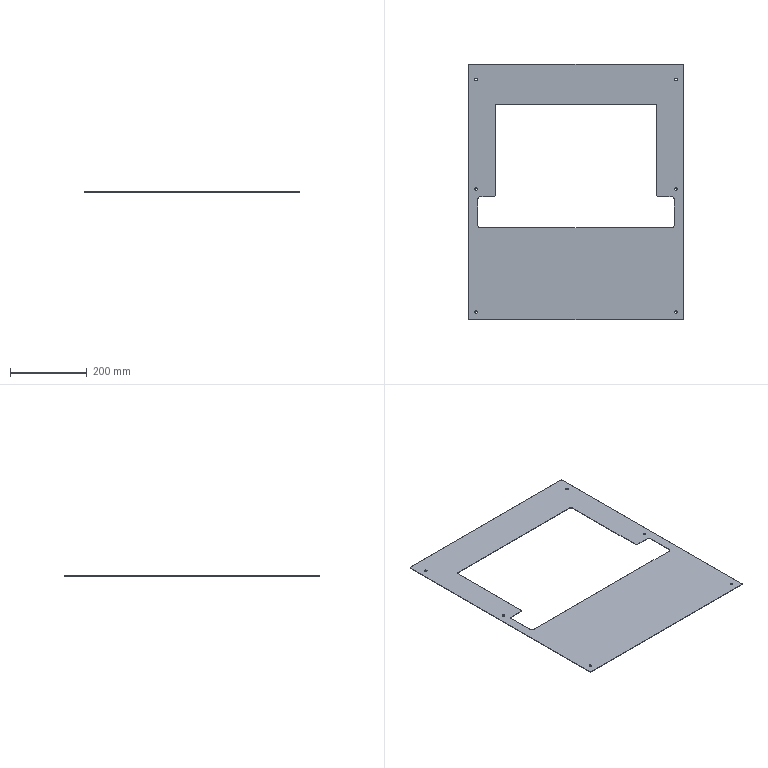Part | SolidWorks | features Fillet 2, ICE 2, FlatPattern 1, HoleWzd 1, SMBaseFlange 1, SheetMetal 1 | 1 solid | 38 faces | box 560 x 665 x 1.2 mm | volume 276730 mm3 | cylinder 24 | plane 14 | commonest cylinder face diameters 6.6 x12 10 x8 6 x4
STEP:
#1=CARTESIAN_POINT('',(16.7,-40.,0.));
#2=VERTEX_POINT('',#1);
#3=CARTESIAN_POINT('',(23.3,-40.,0.));
#4=VERTEX_POINT('',#3);
#5=CARTESIAN_POINT('',(20.,-40.,0.));
#6=DIRECTION('',(0.,0.,1.));
#7=DIRECTION('',(1.,0.,0.));
#8=AXIS2_PLACEMENT_3D('',#5,#6,#7);
#9=CIRCLE('',#8,3.3);
#10=EDGE_CURVE('',#2,#4,#9,.T.);
#11=ORIENTED_EDGE('',*,*,#10,.F.);
#12=CARTESIAN_POINT('',(16.7,-40.,1.2));
#13=VERTEX_POINT('',#12);
#14=CARTESIAN_POINT('',(16.7,-40.,1.2));
#15=DIRECTION('',(0.,0.,1.));
#16=VECTOR('',#15,1000.);
#17=LINE('',#14,#16);
#18=EDGE_CURVE('',#2,#13,#17,.T.);
#19=ORIENTED_EDGE('',*,*,#18,.T.);
#20=CARTESIAN_POINT('',(23.3,-40.,1.2));
#21=VERTEX_POINT('',#20);
#22=CARTESIAN_POINT('',(20.,-40.,1.2));
#23=DIRECTION('',(0.,0.,1.));
#24=DIRECTION('',(1.,0.,0.));
#25=AXIS2_PLACEMENT_3D('',#22,#23,#24);
#26=CIRCLE('',#25,3.3);
#27=EDGE_CURVE('',#13,#21,#26,.T.);
#28=ORIENTED_EDGE('',*,*,#27,.T.);
#29=CARTESIAN_POINT('',(23.3,-40.,1.2));
#30=DIRECTION('',(0.,0.,1.));
#31=VECTOR('',#30,1000.);
#32=LINE('',#29,#31);
#33=EDGE_CURVE('',#4,#21,#32,.T.);
#34=ORIENTED_EDGE('',*,*,#33,.F.);
#35=EDGE_LOOP('',(#11,#19,#28,#34));
#36=FACE_OUTER_BOUND('',#35,.T.);
#37=CARTESIAN_POINT('',(20.,-40.,1.2));
#38=DIRECTION('',(0.,0.,1.));
#39=DIRECTION('',(1.,0.,0.));
#40=AXIS2_PLACEMENT_3D('',#37,#38,#39);
#41=CYLINDRICAL_SURFACE('',#40,3.3);
#42=ADVANCED_FACE('',(#36),#41,.F.);
#43=CARTESIAN_POINT('',(536.7,-40.,0.));
#44=VERTEX_POINT('',#43);
#45=CARTESIAN_POINT('',(543.3,-40.,0.));
#46=VERTEX_POINT('',#45);
#47=CARTESIAN_POINT('',(540.,-40.,0.));
#48=DIRECTION('',(0.,0.,1.));
#49=DIRECTION('',(1.,0.,0.));
#50=AXIS2_PLACEMENT_3D('',#47,#48,#49);
#51=CIRCLE('',#50,3.3);
#52=EDGE_CURVE('',#44,#46,#51,.T.);
#53=ORIENTED_EDGE('',*,*,#52,.F.);
#54=CARTESIAN_POINT('',(536.7,-40.,1.2));
#55=VERTEX_POINT('',#54);
#56=CARTESIAN_POINT('',(536.7,-40.,1.2));
#57=DIRECTION('',(0.,0.,1.));
#58=VECTOR('',#57,1000.);
#59=LINE('',#56,#58);
#60=EDGE_CURVE('',#44,#55,#59,.T.);
#61=ORIENTED_EDGE('',*,*,#60,.T.);
#62=CARTESIAN_POINT('',(543.3,-40.,1.2));
#63=VERTEX_POINT('',#62);
#64=CARTESIAN_POINT('',(540.,-40.,1.2));
#65=DIRECTION('',(0.,0.,1.));
#66=DIRECTION('',(1.,0.,0.));
#67=AXIS2_PLACEMENT_3D('',#64,#65,#66);
#68=CIRCLE('',#67,3.3);
#69=EDGE_CURVE('',#55,#63,#68,.T.);
#70=ORIENTED_EDGE('',*,*,#69,.T.);
#71=CARTESIAN_POINT('',(543.3,-40.,1.2));
#72=DIRECTION('',(0.,0.,1.));
#73=VECTOR('',#72,1000.);
#74=LINE('',#71,#73);
#75=EDGE_CURVE('',#46,#63,#74,.T.);
#76=ORIENTED_EDGE('',*,*,#75,.F.);
#77=EDGE_LOOP('',(#53,#61,#70,#76));
#78=FACE_OUTER_BOUND('',#77,.T.);
#79=CARTESIAN_POINT('',(540.,-40.,1.2));
#80=DIRECTION('',(0.,0.,1.));
#81=DIRECTION('',(1.,0.,0.));
#82=AXIS2_PLACEMENT_3D('',#79,#80,#81);
#83=CYLINDRICAL_SURFACE('',#82,3.3);
#84=ADVANCED_FACE('',(#78),#83,.F.);
#85=CARTESIAN_POINT('',(16.7,-325.,0.));
#86=VERTEX_POINT('',#85);
#87=CARTESIAN_POINT('',(23.3,-325.,0.));
#88=VERTEX_POINT('',#87);
#89=CARTESIAN_POINT('',(20.,-325.,0.));
#90=DIRECTION('',(0.,0.,1.));
#91=DIRECTION('',(1.,0.,0.));
#92=AXIS2_PLACEMENT_3D('',#89,#90,#91);
#93=CIRCLE('',#92,3.3);
#94=EDGE_CURVE('',#86,#88,#93,.T.);
#95=ORIENTED_EDGE('',*,*,#94,.F.);
#96=CARTESIAN_POINT('',(16.7,-325.,1.2));
#97=VERTEX_POINT('',#96);
#98=CARTESIAN_POINT('',(16.7,-325.,1.2));
#99=DIRECTION('',(0.,0.,1.));
#100=VECTOR('',#99,1000.);
#101=LINE('',#98,#100);
#102=EDGE_CURVE('',#86,#97,#101,.T.);
#103=ORIENTED_EDGE('',*,*,#102,.T.);
#104=CARTESIAN_POINT('',(23.3,-325.,1.2));
#105=VERTEX_POINT('',#104);
#106=CARTESIAN_POINT('',(20.,-325.,1.2));
#107=DIRECTION('',(0.,0.,1.));
#108=DIRECTION('',(1.,0.,0.));
#109=AXIS2_PLACEMENT_3D('',#106,#107,#108);
#110=CIRCLE('',#109,3.3);
#111=EDGE_CURVE('',#97,#105,#110,.T.);
#112=ORIENTED_EDGE('',*,*,#111,.T.);
#113=CARTESIAN_POINT('',(23.3,-325.,1.2));
#114=DIRECTION('',(0.,0.,1.));
#115=VECTOR('',#114,1000.);
#116=LINE('',#113,#115);
#117=EDGE_CURVE('',#88,#105,#116,.T.);
#118=ORIENTED_EDGE('',*,*,#117,.F.);
#119=EDGE_LOOP('',(#95,#103,#112,#118));
#120=FACE_OUTER_BOUND('',#119,.T.);
#121=CARTESIAN_POINT('',(20.,-325.,1.2));
#122=DIRECTION('',(0.,0.,1.));
#123=DIRECTION('',(1.,0.,0.));
#124=AXIS2_PLACEMENT_3D('',#121,#122,#123);
#125=CYLINDRICAL_SURFACE('',#124,3.3);
#126=ADVANCED_FACE('',(#120),#125,.F.);
#127=CARTESIAN_POINT('',(536.7,-325.,0.));
#128=VERTEX_POINT('',#127);
#129=CARTESIAN_POINT('',(543.3,-325.,0.));
#130=VERTEX_POINT('',#129);
#131=CARTESIAN_POINT('',(540.,-325.,0.));
#132=DIRECTION('',(0.,0.,1.));
#133=DIRECTION('',(1.,0.,0.));
#134=AXIS2_PLACEMENT_3D('',#131,#132,#133);
#135=CIRCLE('',#134,3.3);
#136=EDGE_CURVE('',#128,#130,#135,.T.);
#137=ORIENTED_EDGE('',*,*,#136,.F.);
#138=CARTESIAN_POINT('',(536.7,-325.,1.2));
#139=VERTEX_POINT('',#138);
#140=CARTESIAN_POINT('',(536.7,-325.,1.2));
#141=DIRECTION('',(0.,0.,1.));
#142=VECTOR('',#141,1000.);
#143=LINE('',#140,#142);
#144=EDGE_CURVE('',#128,#139,#143,.T.);
#145=ORIENTED_EDGE('',*,*,#144,.T.);
#146=CARTESIAN_POINT('',(543.3,-325.,1.2));
#147=VERTEX_POINT('',#146);
#148=CARTESIAN_POINT('',(540.,-325.,1.2));
#149=DIRECTION('',(0.,0.,1.));
#150=DIRECTION('',(1.,0.,0.));
#151=AXIS2_PLACEMENT_3D('',#148,#149,#150);
#152=CIRCLE('',#151,3.3);
#153=EDGE_CURVE('',#139,#147,#152,.T.);
#154=ORIENTED_EDGE('',*,*,#153,.T.);
#155=CARTESIAN_POINT('',(543.3,-325.,1.2));
#156=DIRECTION('',(0.,0.,1.));
#157=VECTOR('',#156,1000.);
#158=LINE('',#155,#157);
#159=EDGE_CURVE('',#130,#147,#158,.T.);
#160=ORIENTED_EDGE('',*,*,#159,.F.);
#161=EDGE_LOOP('',(#137,#145,#154,#160));
#162=FACE_OUTER_BOUND('',#161,.T.);
#163=CARTESIAN_POINT('',(540.,-325.,1.2));
#164=DIRECTION('',(0.,0.,1.));
#165=DIRECTION('',(1.,0.,0.));
#166=AXIS2_PLACEMENT_3D('',#163,#164,#165);
#167=CYLINDRICAL_SURFACE('',#166,3.3);
#168=ADVANCED_FACE('',(#162),#167,.F.);
#169=CARTESIAN_POINT('',(16.7,-645.,0.));
#170=VERTEX_POINT('',#169);
#171=CARTESIAN_POINT('',(23.3,-645.,0.));
#172=VERTEX_POINT('',#171);
#173=CARTESIAN_POINT('',(20.,-645.,0.));
#174=DIRECTION('',(0.,0.,1.));
#175=DIRECTION('',(1.,0.,0.));
#176=AXIS2_PLACEMENT_3D('',#173,#174,#175);
#177=CIRCLE('',#176,3.3);
#178=EDGE_CURVE('',#170,#172,#177,.T.);
#179=ORIENTED_EDGE('',*,*,#178,.F.);
#180=CARTESIAN_POINT('',(16.7,-645.,1.2));
#181=VERTEX_POINT('',#180);
#182=CARTESIAN_POINT('',(16.7,-645.,1.2));
#183=DIRECTION('',(0.,0.,1.));
#184=VECTOR('',#183,1000.);
#185=LINE('',#182,#184);
#186=EDGE_CURVE('',#170,#181,#185,.T.);
#187=ORIENTED_EDGE('',*,*,#186,.T.);
#188=CARTESIAN_POINT('',(23.3,-645.,1.2));
#189=VERTEX_POINT('',#188);
#190=CARTESIAN_POINT('',(20.,-645.,1.2));
#191=DIRECTION('',(0.,0.,1.));
#192=DIRECTION('',(1.,0.,0.));
#193=AXIS2_PLACEMENT_3D('',#190,#191,#192);
#194=CIRCLE('',#193,3.3);
#195=EDGE_CURVE('',#181,#189,#194,.T.);
#196=ORIENTED_EDGE('',*,*,#195,.T.);
#197=CARTESIAN_POINT('',(23.3,-645.,1.2));
#198=DIRECTION('',(0.,0.,1.));
#199=VECTOR('',#198,1000.);
#200=LINE('',#197,#199);
#201=EDGE_CURVE('',#172,#189,#200,.T.);
#202=ORIENTED_EDGE('',*,*,#201,.F.);
#203=EDGE_LOOP('',(#179,#187,#196,#202));
#204=FACE_OUTER_BOUND('',#203,.T.);
#205=CARTESIAN_POINT('',(20.,-645.,1.2));
#206=DIRECTION('',(0.,0.,1.));
#207=DIRECTION('',(1.,0.,0.));
#208=AXIS2_PLACEMENT_3D('',#205,#206,#207);
#209=CYLINDRICAL_SURFACE('',#208,3.3);
#210=ADVANCED_FACE('',(#204),#209,.F.);
#211=CARTESIAN_POINT('',(536.7,-645.,0.));
#212=VERTEX_POINT('',#211);
#213=CARTESIAN_POINT('',(543.3,-645.,0.));
#214=VERTEX_POINT('',#213);
#215=CARTESIAN_POINT('',(540.,-645.,0.));
#216=DIRECTION('',(0.,0.,1.));
#217=DIRECTION('',(1.,0.,0.));
#218=AXIS2_PLACEMENT_3D('',#215,#216,#217);
#219=CIRCLE('',#218,3.3);
#220=EDGE_CURVE('',#212,#214,#219,.T.);
#221=ORIENTED_EDGE('',*,*,#220,.F.);
#222=CARTESIAN_POINT('',(536.7,-645.,1.2));
#223=VERTEX_POINT('',#222);
#224=CARTESIAN_POINT('',(536.7,-645.,1.2));
#225=DIRECTION('',(0.,0.,1.));
#226=VECTOR('',#225,1000.);
#227=LINE('',#224,#226);
#228=EDGE_CURVE('',#212,#223,#227,.T.);
#229=ORIENTED_EDGE('',*,*,#228,.T.);
#230=CARTESIAN_POINT('',(543.3,-645.,1.2));
#231=VERTEX_POINT('',#230);
#232=CARTESIAN_POINT('',(540.,-645.,1.2));
#233=DIRECTION('',(0.,0.,1.));
#234=DIRECTION('',(1.,0.,0.));
#235=AXIS2_PLACEMENT_3D('',#232,#233,#234);
#236=CIRCLE('',#235,3.3);
#237=EDGE_CURVE('',#223,#231,#236,.T.);
#238=ORIENTED_EDGE('',*,*,#237,.T.);
#239=CARTESIAN_POINT('',(543.3,-645.,1.2));
#240=DIRECTION('',(0.,0.,1.));
#241=VECTOR('',#240,1000.);
#242=LINE('',#239,#241);
#243=EDGE_CURVE('',#214,#231,#242,.T.);
#244=ORIENTED_EDGE('',*,*,#243,.F.);
#245=EDGE_LOOP('',(#221,#229,#238,#244));
#246=FACE_OUTER_BOUND('',#245,.T.);
#247=CARTESIAN_POINT('',(540.,-645.,1.2));
#248=DIRECTION('',(0.,0.,1.));
#249=DIRECTION('',(1.,0.,0.));
#250=AXIS2_PLACEMENT_3D('',#247,#248,#249);
#251=CYLINDRICAL_SURFACE('',#250,3.3);
#252=ADVANCED_FACE('',(#246),#251,.F.);
#253=CARTESIAN_POINT('',(0.,-662.,1.2));
#254=VERTEX_POINT('',#253);
#255=CARTESIAN_POINT('',(0.,-3.,1.2));
#256=VERTEX_POINT('',#255);
#257=CARTESIAN_POINT('',(0.,0.,1.2));
#258=DIRECTION('',(0.,1.,0.));
#259=VECTOR('',#258,1000.);
#260=LINE('',#257,#259);
#261=EDGE_CURVE('',#254,#256,#260,.T.);
#262=ORIENTED_EDGE('',*,*,#261,.T.);
#263=CARTESIAN_POINT('',(0.,-3.,0.));
#264=VERTEX_POINT('',#263);
#265=CARTESIAN_POINT('',(0.,-3.,1.2));
#266=DIRECTION('',(0.,0.,-1.));
#267=VECTOR('',#266,1000.);
#268=LINE('',#265,#267);
#269=EDGE_CURVE('',#256,#264,#268,.T.);
#270=ORIENTED_EDGE('',*,*,#269,.T.);
#271=CARTESIAN_POINT('',(0.,-662.,0.));
#272=VERTEX_POINT('',#271);
#273=CARTESIAN_POINT('',(0.,0.,0.));
#274=DIRECTION('',(0.,1.,0.));
#275=VECTOR('',#274,1000.);
#276=LINE('',#273,#275);
#277=EDGE_CURVE('',#272,#264,#276,.T.);
#278=ORIENTED_EDGE('',*,*,#277,.F.);
#279=CARTESIAN_POINT('',(0.,-662.,1.2));
#280=DIRECTION('',(0.,0.,1.));
#281=VECTOR('',#280,1000.);
#282=LINE('',#279,#281);
#283=EDGE_CURVE('',#272,#254,#282,.T.);
#284=ORIENTED_EDGE('',*,*,#283,.T.);
#285=EDGE_LOOP('',(#262,#270,#278,#284));
#286=FACE_OUTER_BOUND('',#285,.T.);
#287=CARTESIAN_POINT('',(0.,0.,1.2));
#288=DIRECTION('',(-1.,0.,0.));
#289=DIRECTION('',(0.,0.,1.));
#290=AXIS2_PLACEMENT_3D('',#287,#288,#289);
#291=PLANE('',#290);
#292=ADVANCED_FACE('',(#286),#291,.T.);
#293=CARTESIAN_POINT('',(557.,-665.,0.));
#294=VERTEX_POINT('',#293);
#295=CARTESIAN_POINT('',(3.,-665.,0.));
#296=VERTEX_POINT('',#295);
#297=CARTESIAN_POINT('',(0.,-665.,0.));
#298=DIRECTION('',(-1.,0.,0.));
#299=VECTOR('',#298,1000.);
#300=LINE('',#297,#299);
#301=EDGE_CURVE('',#294,#296,#300,.T.);
#302=ORIENTED_EDGE('',*,*,#301,.F.);
#303=CARTESIAN_POINT('',(557.,-665.,1.2));
#304=VERTEX_POINT('',#303);
#305=CARTESIAN_POINT('',(557.,-665.,1.2));
#306=DIRECTION('',(0.,0.,1.));
#307=VECTOR('',#306,1000.);
#308=LINE('',#305,#307);
#309=EDGE_CURVE('',#294,#304,#308,.T.);
#310=ORIENTED_EDGE('',*,*,#309,.T.);
#311=CARTESIAN_POINT('',(3.,-665.,1.2));
#312=VERTEX_POINT('',#311);
#313=CARTESIAN_POINT('',(0.,-665.,1.2));
#314=DIRECTION('',(-1.,0.,0.));
#315=VECTOR('',#314,1000.);
#316=LINE('',#313,#315);
#317=EDGE_CURVE('',#304,#312,#316,.T.);
#318=ORIENTED_EDGE('',*,*,#317,.T.);
#319=CARTESIAN_POINT('',(3.,-665.,1.2));
#320=DIRECTION('',(0.,0.,-1.));
#321=VECTOR('',#320,1000.);
#322=LINE('',#319,#321);
#323=EDGE_CURVE('',#312,#296,#322,.T.);
#324=ORIENTED_EDGE('',*,*,#323,.T.);
#325=EDGE_LOOP('',(#302,#310,#318,#324));
#326=FACE_OUTER_BOUND('',#325,.T.);
#327=CARTESIAN_POINT('',(0.,-665.,1.2));
#328=DIRECTION('',(0.,-1.,0.));
#329=DIRECTION('',(0.,0.,-1.));
#330=AXIS2_PLACEMENT_3D('',#327,#328,#329);
#331=PLANE('',#330);
#332=ADVANCED_FACE('',(#326),#331,.T.);
#333=CARTESIAN_POINT('',(560.,-3.,0.));
#334=VERTEX_POINT('',#333);
#335=CARTESIAN_POINT('',(560.,-662.,0.));
#336=VERTEX_POINT('',#335);
#337=CARTESIAN_POINT('',(560.,0.,0.));
#338=DIRECTION('',(0.,-1.,0.));
#339=VECTOR('',#338,1000.);
#340=LINE('',#337,#339);
#341=EDGE_CURVE('',#334,#336,#340,.T.);
#342=ORIENTED_EDGE('',*,*,#341,.F.);
#343=CARTESIAN_POINT('',(560.,-3.,1.2));
#344=VERTEX_POINT('',#343);
#345=CARTESIAN_POINT('',(560.,-3.,1.2));
#346=DIRECTION('',(0.,0.,1.));
#347=VECTOR('',#346,1000.);
#348=LINE('',#345,#347);
#349=EDGE_CURVE('',#334,#344,#348,.T.);
#350=ORIENTED_EDGE('',*,*,#349,.T.);
#351=CARTESIAN_POINT('',(560.,-662.,1.2));
#352=VERTEX_POINT('',#351);
#353=CARTESIAN_POINT('',(560.,0.,1.2));
#354=DIRECTION('',(0.,-1.,0.));
#355=VECTOR('',#354,1000.);
#356=LINE('',#353,#355);
#357=EDGE_CURVE('',#344,#352,#356,.T.);
#358=ORIENTED_EDGE('',*,*,#357,.T.);
#359=CARTESIAN_POINT('',(560.,-662.,1.2));
#360=DIRECTION('',(0.,0.,-1.));
#361=VECTOR('',#360,1000.);
#362=LINE('',#359,#361);
#363=EDGE_CURVE('',#352,#336,#362,.T.);
#364=ORIENTED_EDGE('',*,*,#363,.T.);
#365=EDGE_LOOP('',(#342,#350,#358,#364));
#366=FACE_OUTER_BOUND('',#365,.T.);
#367=CARTESIAN_POINT('',(560.,0.,1.2));
#368=DIRECTION('',(1.,0.,0.));
#369=DIRECTION('',(0.,0.,-1.));
#370=AXIS2_PLACEMENT_3D('',#367,#368,#369);
#371=PLANE('',#370);
#372=ADVANCED_FACE('',(#366),#371,.T.);
#373=CARTESIAN_POINT('',(3.,0.,1.2));
#374=VERTEX_POINT('',#373);
#375=CARTESIAN_POINT('',(557.,0.,1.2));
#376=VERTEX_POINT('',#375);
#377=CARTESIAN_POINT('',(0.,0.,1.2));
#378=DIRECTION('',(1.,0.,0.));
#379=VECTOR('',#378,1000.);
#380=LINE('',#377,#379);
#381=EDGE_CURVE('',#374,#376,#380,.T.);
#382=ORIENTED_EDGE('',*,*,#381,.T.);
#383=CARTESIAN_POINT('',(557.,0.,0.));
#384=VERTEX_POINT('',#383);
#385=CARTESIAN_POINT('',(557.,0.,1.2));
#386=DIRECTION('',(0.,0.,-1.));
#387=VECTOR('',#386,1000.);
#388=LINE('',#385,#387);
#389=EDGE_CURVE('',#376,#384,#388,.T.);
#390=ORIENTED_EDGE('',*,*,#389,.T.);
#391=CARTESIAN_POINT('',(3.,0.,0.));
#392=VERTEX_POINT('',#391);
#393=CARTESIAN_POINT('',(0.,0.,0.));
#394=DIRECTION('',(1.,0.,0.));
#395=VECTOR('',#394,1000.);
#396=LINE('',#393,#395);
#397=EDGE_CURVE('',#392,#384,#396,.T.);
#398=ORIENTED_EDGE('',*,*,#397,.F.);
#399=CARTESIAN_POINT('',(3.,0.,1.2));
#400=DIRECTION('',(0.,0.,1.));
#401=VECTOR('',#400,1000.);
#402=LINE('',#399,#401);
#403=EDGE_CURVE('',#392,#374,#402,.T.);
#404=ORIENTED_EDGE('',*,*,#403,.T.);
#405=EDGE_LOOP('',(#382,#390,#398,#404));
#406=FACE_OUTER_BOUND('',#405,.T.);
#407=CARTESIAN_POINT('',(0.,0.,1.2));
#408=DIRECTION('',(0.,1.,0.));
#409=DIRECTION('',(0.,0.,1.));
#410=AXIS2_PLACEMENT_3D('',#407,#408,#409);
#411=PLANE('',#410);
#412=ADVANCED_FACE('',(#406),#411,.T.);
#413=CARTESIAN_POINT('',(20.,-40.,1.2));
#414=DIRECTION('',(0.,0.,1.));
#415=DIRECTION('',(1.,0.,0.));
#416=AXIS2_PLACEMENT_3D('',#413,#414,#415);
#417=CIRCLE('',#416,3.3);
#418=EDGE_CURVE('',#21,#13,#417,.T.);
#419=ORIENTED_EDGE('',*,*,#418,.F.);
#420=ORIENTED_EDGE('',*,*,#27,.F.);
#421=EDGE_LOOP('',(#419,#420));
#422=FACE_BOUND('',#421,.T.);
#423=CARTESIAN_POINT('',(540.,-40.,1.2));
#424=DIRECTION('',(0.,0.,1.));
#425=DIRECTION('',(1.,0.,0.));
#426=AXIS2_PLACEMENT_3D('',#423,#424,#425);
#427=CIRCLE('',#426,3.3);
#428=EDGE_CURVE('',#63,#55,#427,.T.);
#429=ORIENTED_EDGE('',*,*,#428,.F.);
#430=ORIENTED_EDGE('',*,*,#69,.F.);
#431=EDGE_LOOP('',(#429,#430));
#432=FACE_BOUND('',#431,.T.);
#433=CARTESIAN_POINT('',(20.,-325.,1.2));
#434=DIRECTION('',(0.,0.,1.));
#435=DIRECTION('',(1.,0.,0.));
#436=AXIS2_PLACEMENT_3D('',#433,#434,#435);
#437=CIRCLE('',#436,3.3);
#438=EDGE_CURVE('',#105,#97,#437,.T.);
#439=ORIENTED_EDGE('',*,*,#438,.F.);
#440=ORIENTED_EDGE('',*,*,#111,.F.);
#441=EDGE_LOOP('',(#439,#440));
#442=FACE_BOUND('',#441,.T.);
#443=CARTESIAN_POINT('',(540.,-325.,1.2));
#444=DIRECTION('',(0.,0.,1.));
#445=DIRECTION('',(1.,0.,0.));
#446=AXIS2_PLACEMENT_3D('',#443,#444,#445);
#447=CIRCLE('',#446,3.3);
#448=EDGE_CURVE('',#147,#139,#447,.T.);
#449=ORIENTED_EDGE('',*,*,#448,.F.);
#450=ORIENTED_EDGE('',*,*,#153,.F.);
#451=EDGE_LOOP('',(#449,#450));
#452=FACE_BOUND('',#451,.T.);
#453=CARTESIAN_POINT('',(20.,-645.,1.2));
#454=DIRECTION('',(0.,0.,1.));
#455=DIRECTION('',(1.,0.,0.));
#456=AXIS2_PLACEMENT_3D('',#453,#454,#455);
#457=CIRCLE('',#456,3.3);
#458=EDGE_CURVE('',#189,#181,#457,.T.);
#459=ORIENTED_EDGE('',*,*,#458,.F.);
#460=ORIENTED_EDGE('',*,*,#195,.F.);
#461=EDGE_LOOP('',(#459,#460));
#462=FACE_BOUND('',#461,.T.);
#463=CARTESIAN_POINT('',(540.,-645.,1.2));
#464=DIRECTION('',(0.,0.,1.));
#465=DIRECTION('',(1.,0.,0.));
#466=AXIS2_PLACEMENT_3D('',#463,#464,#465);
#467=CIRCLE('',#466,3.3);
#468=EDGE_CURVE('',#231,#223,#467,.T.);
#469=ORIENTED_EDGE('',*,*,#468,.F.);
#470=ORIENTED_EDGE('',*,*,#237,.F.);
#471=EDGE_LOOP('',(#469,#470));
#472=FACE_BOUND('',#471,.T.);
#473=CARTESIAN_POINT('',(65.,-345.,1.2));
#474=VERTEX_POINT('',#473);
#475=CARTESIAN_POINT('',(30.,-345.,1.2));
#476=VERTEX_POINT('',#475);
#477=CARTESIAN_POINT('',(25.,-345.,1.2));
#478=DIRECTION('',(-1.,0.,0.));
#479=VECTOR('',#478,1000.);
#480=LINE('',#477,#479);
#481=EDGE_CURVE('',#474,#476,#480,.T.);
#482=ORIENTED_EDGE('',*,*,#481,.F.);
#483=CARTESIAN_POINT('',(70.,-340.,1.2));
#484=VERTEX_POINT('',#483);
#485=CARTESIAN_POINT('',(65.,-340.,1.2));
#486=DIRECTION('',(0.,0.,1.));
#487=DIRECTION('',(1.,0.,0.));
#488=AXIS2_PLACEMENT_3D('',#485,#486,#487);
#489=CIRCLE('',#488,5.);
#490=EDGE_CURVE('',#474,#484,#489,.T.);
#491=ORIENTED_EDGE('',*,*,#490,.T.);
#492=CARTESIAN_POINT('',(70.,-110.,1.2));
#493=VERTEX_POINT('',#492);
#494=CARTESIAN_POINT('',(70.,-105.,1.2));
#495=DIRECTION('',(0.,-1.,0.));
#496=VECTOR('',#495,1000.);
#497=LINE('',#494,#496);
#498=EDGE_CURVE('',#493,#484,#497,.T.);
#499=ORIENTED_EDGE('',*,*,#498,.F.);
#500=CARTESIAN_POINT('',(75.,-105.,1.2));
#501=VERTEX_POINT('',#500);
#502=CARTESIAN_POINT('',(75.,-110.,1.2));
#503=DIRECTION('',(0.,0.,-1.));
#504=DIRECTION('',(1.,0.,0.));
#505=AXIS2_PLACEMENT_3D('',#502,#503,#504);
#506=CIRCLE('',#505,5.);
#507=EDGE_CURVE('',#493,#501,#506,.T.);
#508=ORIENTED_EDGE('',*,*,#507,.T.);
#509=CARTESIAN_POINT('',(485.,-105.,1.2));
#510=VERTEX_POINT('',#509);
#511=CARTESIAN_POINT('',(70.,-105.,1.2));
#512=DIRECTION('',(-1.,0.,0.));
#513=VECTOR('',#512,1000.);
#514=LINE('',#511,#513);
#515=EDGE_CURVE('',#510,#501,#514,.T.);
#516=ORIENTED_EDGE('',*,*,#515,.F.);
#517=CARTESIAN_POINT('',(490.,-110.,1.2));
#518=VERTEX_POINT('',#517);
#519=CARTESIAN_POINT('',(485.,-110.,1.2));
#520=DIRECTION('',(0.,0.,-1.));
#521=DIRECTION('',(1.,0.,0.));
#522=AXIS2_PLACEMENT_3D('',#519,#520,#521);
#523=CIRCLE('',#522,5.);
#524=EDGE_CURVE('',#510,#518,#523,.T.);
#525=ORIENTED_EDGE('',*,*,#524,.T.);
#526=CARTESIAN_POINT('',(490.,-340.,1.2));
#527=VERTEX_POINT('',#526);
#528=CARTESIAN_POINT('',(490.,-105.,1.2));
#529=DIRECTION('',(0.,1.,0.));
#530=VECTOR('',#529,1000.);
#531=LINE('',#528,#530);
#532=EDGE_CURVE('',#527,#518,#531,.T.);
#533=ORIENTED_EDGE('',*,*,#532,.F.);
#534=CARTESIAN_POINT('',(495.,-345.,1.2));
#535=VERTEX_POINT('',#534);
#536=CARTESIAN_POINT('',(495.,-340.,1.2));
#537=DIRECTION('',(0.,0.,1.));
#538=DIRECTION('',(1.,0.,0.));
#539=AXIS2_PLACEMENT_3D('',#536,#537,#538);
#540=CIRCLE('',#539,5.);
#541=EDGE_CURVE('',#527,#535,#540,.T.);
#542=ORIENTED_EDGE('',*,*,#541,.T.);
#543=CARTESIAN_POINT('',(530.,-345.,1.2));
#544=VERTEX_POINT('',#543);
#545=CARTESIAN_POINT('',(25.,-345.,1.2));
#546=DIRECTION('',(-1.,0.,0.));
#547=VECTOR('',#546,1000.);
#548=LINE('',#545,#547);
#549=EDGE_CURVE('',#544,#535,#548,.T.);
#550=ORIENTED_EDGE('',*,*,#549,.F.);
#551=CARTESIAN_POINT('',(535.,-350.,1.2));
#552=VERTEX_POINT('',#551);
#553=CARTESIAN_POINT('',(530.,-350.,1.2));
#554=DIRECTION('',(0.,0.,-1.));
#555=DIRECTION('',(1.,0.,0.));
#556=AXIS2_PLACEMENT_3D('',#553,#554,#555);
#557=CIRCLE('',#556,5.);
#558=EDGE_CURVE('',#544,#552,#557,.T.);
#559=ORIENTED_EDGE('',*,*,#558,.T.);
#560=CARTESIAN_POINT('',(535.,-420.,1.2));
#561=VERTEX_POINT('',#560);
#562=CARTESIAN_POINT('',(535.,-345.,1.2));
#563=DIRECTION('',(0.,1.,0.));
#564=VECTOR('',#563,1000.);
#565=LINE('',#562,#564);
#566=EDGE_CURVE('',#561,#552,#565,.T.);
#567=ORIENTED_EDGE('',*,*,#566,.F.);
#568=CARTESIAN_POINT('',(530.,-425.,1.2));
#569=VERTEX_POINT('',#568);
#570=CARTESIAN_POINT('',(530.,-420.,1.2));
#571=DIRECTION('',(0.,0.,-1.));
#572=DIRECTION('',(1.,0.,0.));
#573=AXIS2_PLACEMENT_3D('',#570,#571,#572);
#574=CIRCLE('',#573,5.);
#575=EDGE_CURVE('',#561,#569,#574,.T.);
#576=ORIENTED_EDGE('',*,*,#575,.T.);
#577=CARTESIAN_POINT('',(30.,-425.,1.2));
#578=VERTEX_POINT('',#577);
#579=CARTESIAN_POINT('',(70.,-425.,1.2));
#580=DIRECTION('',(1.,0.,0.));
#581=VECTOR('',#580,1000.);
#582=LINE('',#579,#581);
#583=EDGE_CURVE('',#578,#569,#582,.T.);
#584=ORIENTED_EDGE('',*,*,#583,.F.);
#585=CARTESIAN_POINT('',(25.,-420.,1.2));
#586=VERTEX_POINT('',#585);
#587=CARTESIAN_POINT('',(30.,-420.,1.2));
#588=DIRECTION('',(0.,0.,-1.));
#589=DIRECTION('',(1.,0.,0.));
#590=AXIS2_PLACEMENT_3D('',#587,#588,#589);
#591=CIRCLE('',#590,5.);
#592=EDGE_CURVE('',#578,#586,#591,.T.);
#593=ORIENTED_EDGE('',*,*,#592,.T.);
#594=CARTESIAN_POINT('',(25.,-350.,1.2));
#595=VERTEX_POINT('',#594);
#596=CARTESIAN_POINT('',(25.,-345.,1.2));
#597=DIRECTION('',(0.,-1.,0.));
#598=VECTOR('',#597,1000.);
#599=LINE('',#596,#598);
#600=EDGE_CURVE('',#595,#586,#599,.T.);
#601=ORIENTED_EDGE('',*,*,#600,.F.);
#602=CARTESIAN_POINT('',(30.,-350.,1.2));
#603=DIRECTION('',(0.,0.,-1.));
#604=DIRECTION('',(1.,0.,0.));
#605=AXIS2_PLACEMENT_3D('',#602,#603,#604);
#606=CIRCLE('',#605,5.);
#607=EDGE_CURVE('',#595,#476,#606,.T.);
#608=ORIENTED_EDGE('',*,*,#607,.T.);
#609=EDGE_LOOP('',(#482,#491,#499,#508,#516,#525,#533,#542,#550,#559,#567,#576,#584,#593,#601,#608));
#610=FACE_BOUND('',#609,.T.);
#611=ORIENTED_EDGE('',*,*,#357,.F.);
#612=CARTESIAN_POINT('',(557.,-3.,1.2));
#613=DIRECTION('',(0.,0.,1.));
#614=DIRECTION('',(1.,0.,0.));
#615=AXIS2_PLACEMENT_3D('',#612,#613,#614);
#616=CIRCLE('',#615,3.);
#617=EDGE_CURVE('',#344,#376,#616,.T.);
#618=ORIENTED_EDGE('',*,*,#617,.T.);
#619=ORIENTED_EDGE('',*,*,#381,.F.);
#620=CARTESIAN_POINT('',(3.,-3.,1.2));
#621=DIRECTION('',(0.,0.,1.));
#622=DIRECTION('',(1.,0.,0.));
#623=AXIS2_PLACEMENT_3D('',#620,#621,#622);
#624=CIRCLE('',#623,3.);
#625=EDGE_CURVE('',#374,#256,#624,.T.);
#626=ORIENTED_EDGE('',*,*,#625,.T.);
#627=ORIENTED_EDGE('',*,*,#261,.F.);
#628=CARTESIAN_POINT('',(3.,-662.,1.2));
#629=DIRECTION('',(0.,0.,1.));
#630=DIRECTION('',(1.,0.,0.));
#631=AXIS2_PLACEMENT_3D('',#628,#629,#630);
#632=CIRCLE('',#631,3.);
#633=EDGE_CURVE('',#254,#312,#632,.T.);
#634=ORIENTED_EDGE('',*,*,#633,.T.);
#635=ORIENTED_EDGE('',*,*,#317,.F.);
#636=CARTESIAN_POINT('',(557.,-662.,1.2));
#637=DIRECTION('',(0.,0.,1.));
#638=DIRECTION('',(1.,0.,0.));
#639=AXIS2_PLACEMENT_3D('',#636,#637,#638);
#640=CIRCLE('',#639,3.);
#641=EDGE_CURVE('',#304,#352,#640,.T.);
#642=ORIENTED_EDGE('',*,*,#641,.T.);
#643=EDGE_LOOP('',(#611,#618,#619,#626,#627,#634,#635,#642));
#644=FACE_OUTER_BOUND('',#643,.T.);
#645=CARTESIAN_POINT('',(0.,0.,1.2));
#646=DIRECTION('',(0.,0.,1.));
#647=DIRECTION('',(1.,0.,0.));
#648=AXIS2_PLACEMENT_3D('',#645,#646,#647);
#649=PLANE('',#648);
#650=ADVANCED_FACE('',(#422,#432,#442,#452,#462,#472,#610,#644),#649,.T.);
#651=CARTESIAN_POINT('',(20.,-40.,0.));
#652=DIRECTION('',(0.,0.,1.));
#653=DIRECTION('',(1.,0.,0.));
#654=AXIS2_PLACEMENT_3D('',#651,#652,#653);
#655=CIRCLE('',#654,3.3);
#656=EDGE_CURVE('',#4,#2,#655,.T.);
#657=ORIENTED_EDGE('',*,*,#656,.T.);
#658=ORIENTED_EDGE('',*,*,#10,.T.);
#659=EDGE_LOOP('',(#657,#658));
#660=FACE_BOUND('',#659,.T.);
#661=CARTESIAN_POINT('',(540.,-40.,0.));
#662=DIRECTION('',(0.,0.,1.));
#663=DIRECTION('',(1.,0.,0.));
#664=AXIS2_PLACEMENT_3D('',#661,#662,#663);
#665=CIRCLE('',#664,3.3);
#666=EDGE_CURVE('',#46,#44,#665,.T.);
#667=ORIENTED_EDGE('',*,*,#666,.T.);
#668=ORIENTED_EDGE('',*,*,#52,.T.);
#669=EDGE_LOOP('',(#667,#668));
#670=FACE_BOUND('',#669,.T.);
#671=CARTESIAN_POINT('',(20.,-325.,0.));
#672=DIRECTION('',(0.,0.,1.));
#673=DIRECTION('',(1.,0.,0.));
#674=AXIS2_PLACEMENT_3D('',#671,#672,#673);
#675=CIRCLE('',#674,3.3);
#676=EDGE_CURVE('',#88,#86,#675,.T.);
#677=ORIENTED_EDGE('',*,*,#676,.T.);
#678=ORIENTED_EDGE('',*,*,#94,.T.);
#679=EDGE_LOOP('',(#677,#678));
#680=FACE_BOUND('',#679,.T.);
#681=CARTESIAN_POINT('',(540.,-325.,0.));
#682=DIRECTION('',(0.,0.,1.));
#683=DIRECTION('',(1.,0.,0.));
#684=AXIS2_PLACEMENT_3D('',#681,#682,#683);
#685=CIRCLE('',#684,3.3);
#686=EDGE_CURVE('',#130,#128,#685,.T.);
#687=ORIENTED_EDGE('',*,*,#686,.T.);
#688=ORIENTED_EDGE('',*,*,#136,.T.);
#689=EDGE_LOOP('',(#687,#688));
#690=FACE_BOUND('',#689,.T.);
#691=CARTESIAN_POINT('',(20.,-645.,0.));
#692=DIRECTION('',(0.,0.,1.));
#693=DIRECTION('',(1.,0.,0.));
#694=AXIS2_PLACEMENT_3D('',#691,#692,#693);
#695=CIRCLE('',#694,3.3);
#696=EDGE_CURVE('',#172,#170,#695,.T.);
#697=ORIENTED_EDGE('',*,*,#696,.T.);
#698=ORIENTED_EDGE('',*,*,#178,.T.);
#699=EDGE_LOOP('',(#697,#698));
#700=FACE_BOUND('',#699,.T.);
#701=CARTESIAN_POINT('',(540.,-645.,0.));
#702=DIRECTION('',(0.,0.,1.));
#703=DIRECTION('',(1.,0.,0.));
#704=AXIS2_PLACEMENT_3D('',#701,#702,#703);
#705=CIRCLE('',#704,3.3);
#706=EDGE_CURVE('',#214,#212,#705,.T.);
#707=ORIENTED_EDGE('',*,*,#706,.T.);
#708=ORIENTED_EDGE('',*,*,#220,.T.);
#709=EDGE_LOOP('',(#707,#708));
#710=FACE_BOUND('',#709,.T.);
#711=CARTESIAN_POINT('',(70.,-110.,0.));
#712=VERTEX_POINT('',#711);
#713=CARTESIAN_POINT('',(70.,-340.,0.));
#714=VERTEX_POINT('',#713);
#715=CARTESIAN_POINT('',(70.,0.,0.));
#716=DIRECTION('',(0.,-1.,0.));
#717=VECTOR('',#716,1000.);
#718=LINE('',#715,#717);
#719=EDGE_CURVE('',#712,#714,#718,.T.);
#720=ORIENTED_EDGE('',*,*,#719,.T.);
#721=CARTESIAN_POINT('',(65.,-345.,0.));
#722=VERTEX_POINT('',#721);
#723=CARTESIAN_POINT('',(65.,-340.,0.));
#724=DIRECTION('',(0.,0.,-1.));
#725=DIRECTION('',(1.,0.,0.));
#726=AXIS2_PLACEMENT_3D('',#723,#724,#725);
#727=CIRCLE('',#726,5.);
#728=EDGE_CURVE('',#714,#722,#727,.T.);
#729=ORIENTED_EDGE('',*,*,#728,.T.);
#730=CARTESIAN_POINT('',(30.,-345.,0.));
#731=VERTEX_POINT('',#730);
#732=CARTESIAN_POINT('',(0.,-345.,0.));
#733=DIRECTION('',(-1.,0.,0.));
#734=VECTOR('',#733,1000.);
#735=LINE('',#732,#734);
#736=EDGE_CURVE('',#722,#731,#735,.T.);
#737=ORIENTED_EDGE('',*,*,#736,.T.);
#738=CARTESIAN_POINT('',(25.,-350.,0.));
#739=VERTEX_POINT('',#738);
#740=CARTESIAN_POINT('',(30.,-350.,0.));
#741=DIRECTION('',(0.,0.,1.));
#742=DIRECTION('',(1.,0.,0.));
#743=AXIS2_PLACEMENT_3D('',#740,#741,#742);
#744=CIRCLE('',#743,5.);
#745=EDGE_CURVE('',#731,#739,#744,.T.);
#746=ORIENTED_EDGE('',*,*,#745,.T.);
#747=CARTESIAN_POINT('',(25.,-420.,0.));
#748=VERTEX_POINT('',#747);
#749=CARTESIAN_POINT('',(25.,0.,0.));
#750=DIRECTION('',(0.,-1.,0.));
#751=VECTOR('',#750,1000.);
#752=LINE('',#749,#751);
#753=EDGE_CURVE('',#739,#748,#752,.T.);
#754=ORIENTED_EDGE('',*,*,#753,.T.);
#755=CARTESIAN_POINT('',(30.,-425.,0.));
#756=VERTEX_POINT('',#755);
#757=CARTESIAN_POINT('',(30.,-420.,0.));
#758=DIRECTION('',(0.,0.,1.));
#759=DIRECTION('',(1.,0.,0.));
#760=AXIS2_PLACEMENT_3D('',#757,#758,#759);
#761=CIRCLE('',#760,5.);
#762=EDGE_CURVE('',#748,#756,#761,.T.);
#763=ORIENTED_EDGE('',*,*,#762,.T.);
#764=CARTESIAN_POINT('',(530.,-425.,0.));
#765=VERTEX_POINT('',#764);
#766=CARTESIAN_POINT('',(0.,-425.,0.));
#767=DIRECTION('',(1.,0.,0.));
#768=VECTOR('',#767,1000.);
#769=LINE('',#766,#768);
#770=EDGE_CURVE('',#756,#765,#769,.T.);
#771=ORIENTED_EDGE('',*,*,#770,.T.);
#772=CARTESIAN_POINT('',(535.,-420.,0.));
#773=VERTEX_POINT('',#772);
#774=CARTESIAN_POINT('',(530.,-420.,0.));
#775=DIRECTION('',(0.,0.,1.));
#776=DIRECTION('',(1.,0.,0.));
#777=AXIS2_PLACEMENT_3D('',#774,#775,#776);
#778=CIRCLE('',#777,5.);
#779=EDGE_CURVE('',#765,#773,#778,.T.);
#780=ORIENTED_EDGE('',*,*,#779,.T.);
#781=CARTESIAN_POINT('',(535.,-350.,0.));
#782=VERTEX_POINT('',#781);
#783=CARTESIAN_POINT('',(535.,0.,0.));
#784=DIRECTION('',(0.,1.,0.));
#785=VECTOR('',#784,1000.);
#786=LINE('',#783,#785);
#787=EDGE_CURVE('',#773,#782,#786,.T.);
#788=ORIENTED_EDGE('',*,*,#787,.T.);
#789=CARTESIAN_POINT('',(530.,-345.,0.));
#790=VERTEX_POINT('',#789);
#791=CARTESIAN_POINT('',(530.,-350.,0.));
#792=DIRECTION('',(0.,0.,1.));
#793=DIRECTION('',(1.,0.,0.));
#794=AXIS2_PLACEMENT_3D('',#791,#792,#793);
#795=CIRCLE('',#794,5.);
#796=EDGE_CURVE('',#782,#790,#795,.T.);
#797=ORIENTED_EDGE('',*,*,#796,.T.);
#798=CARTESIAN_POINT('',(495.,-345.,0.));
#799=VERTEX_POINT('',#798);
#800=CARTESIAN_POINT('',(0.,-345.,0.));
#801=DIRECTION('',(-1.,0.,0.));
#802=VECTOR('',#801,1000.);
#803=LINE('',#800,#802);
#804=EDGE_CURVE('',#790,#799,#803,.T.);
#805=ORIENTED_EDGE('',*,*,#804,.T.);
#806=CARTESIAN_POINT('',(490.,-340.,0.));
#807=VERTEX_POINT('',#806);
#808=CARTESIAN_POINT('',(495.,-340.,0.));
#809=DIRECTION('',(0.,0.,-1.));
#810=DIRECTION('',(1.,0.,0.));
#811=AXIS2_PLACEMENT_3D('',#808,#809,#810);
#812=CIRCLE('',#811,5.);
#813=EDGE_CURVE('',#799,#807,#812,.T.);
#814=ORIENTED_EDGE('',*,*,#813,.T.);
#815=CARTESIAN_POINT('',(490.,-110.,0.));
#816=VERTEX_POINT('',#815);
#817=CARTESIAN_POINT('',(490.,0.,0.));
#818=DIRECTION('',(0.,1.,0.));
#819=VECTOR('',#818,1000.);
#820=LINE('',#817,#819);
#821=EDGE_CURVE('',#807,#816,#820,.T.);
#822=ORIENTED_EDGE('',*,*,#821,.T.);
#823=CARTESIAN_POINT('',(485.,-105.,0.));
#824=VERTEX_POINT('',#823);
#825=CARTESIAN_POINT('',(485.,-110.,0.));
#826=DIRECTION('',(0.,0.,1.));
#827=DIRECTION('',(1.,0.,0.));
#828=AXIS2_PLACEMENT_3D('',#825,#826,#827);
#829=CIRCLE('',#828,5.);
#830=EDGE_CURVE('',#816,#824,#829,.T.);
#831=ORIENTED_EDGE('',*,*,#830,.T.);
#832=CARTESIAN_POINT('',(75.,-105.,0.));
#833=VERTEX_POINT('',#832);
#834=CARTESIAN_POINT('',(0.,-105.,0.));
#835=DIRECTION('',(-1.,0.,0.));
#836=VECTOR('',#835,1000.);
#837=LINE('',#834,#836);
#838=EDGE_CURVE('',#824,#833,#837,.T.);
#839=ORIENTED_EDGE('',*,*,#838,.T.);
#840=CARTESIAN_POINT('',(75.,-110.,0.));
#841=DIRECTION('',(0.,0.,1.));
#842=DIRECTION('',(1.,0.,0.));
#843=AXIS2_PLACEMENT_3D('',#840,#841,#842);
#844=CIRCLE('',#843,5.);
#845=EDGE_CURVE('',#833,#712,#844,.T.);
#846=ORIENTED_EDGE('',*,*,#845,.T.);
#847=EDGE_LOOP('',(#720,#729,#737,#746,#754,#763,#771,#780,#788,#797,#805,#814,#822,#831,#839,#846));
#848=FACE_BOUND('',#847,.T.);
#849=ORIENTED_EDGE('',*,*,#397,.T.);
#850=CARTESIAN_POINT('',(557.,-3.,0.));
#851=DIRECTION('',(0.,0.,-1.));
#852=DIRECTION('',(1.,0.,0.));
#853=AXIS2_PLACEMENT_3D('',#850,#851,#852);
#854=CIRCLE('',#853,3.);
#855=EDGE_CURVE('',#384,#334,#854,.T.);
#856=ORIENTED_EDGE('',*,*,#855,.T.);
#857=ORIENTED_EDGE('',*,*,#341,.T.);
#858=CARTESIAN_POINT('',(557.,-662.,0.));
#859=DIRECTION('',(0.,0.,-1.));
#860=DIRECTION('',(1.,0.,0.));
#861=AXIS2_PLACEMENT_3D('',#858,#859,#860);
#862=CIRCLE('',#861,3.);
#863=EDGE_CURVE('',#336,#294,#862,.T.);
#864=ORIENTED_EDGE('',*,*,#863,.T.);
#865=ORIENTED_EDGE('',*,*,#301,.T.);
#866=CARTESIAN_POINT('',(3.,-662.,0.));
#867=DIRECTION('',(0.,0.,-1.));
#868=DIRECTION('',(1.,0.,0.));
#869=AXIS2_PLACEMENT_3D('',#866,#867,#868);
#870=CIRCLE('',#869,3.);
#871=EDGE_CURVE('',#296,#272,#870,.T.);
#872=ORIENTED_EDGE('',*,*,#871,.T.);
#873=ORIENTED_EDGE('',*,*,#277,.T.);
#874=CARTESIAN_POINT('',(3.,-3.,0.));
#875=DIRECTION('',(0.,0.,-1.));
#876=DIRECTION('',(1.,0.,0.));
#877=AXIS2_PLACEMENT_3D('',#874,#875,#876);
#878=CIRCLE('',#877,3.);
#879=EDGE_CURVE('',#264,#392,#878,.T.);
#880=ORIENTED_EDGE('',*,*,#879,.T.);
#881=EDGE_LOOP('',(#849,#856,#857,#864,#865,#872,#873,#880));
#882=FACE_OUTER_BOUND('',#881,.T.);
#883=CARTESIAN_POINT('',(0.,0.,0.));
#884=DIRECTION('',(0.,0.,1.));
#885=DIRECTION('',(1.,0.,0.));
#886=AXIS2_PLACEMENT_3D('',#883,#884,#885);
#887=PLANE('',#886);
#888=ADVANCED_FACE('',(#660,#670,#680,#690,#700,#710,#848,#882),#887,.F.);
#889=ORIENTED_EDGE('',*,*,#498,.T.);
#890=CARTESIAN_POINT('',(70.,-340.,-8.8));
#891=DIRECTION('',(0.,0.,-1.));
#892=VECTOR('',#891,1000.);
#893=LINE('',#890,#892);
#894=EDGE_CURVE('',#484,#714,#893,.T.);
#895=ORIENTED_EDGE('',*,*,#894,.T.);
#896=ORIENTED_EDGE('',*,*,#719,.F.);
#897=CARTESIAN_POINT('',(70.,-110.,1.2));
#898=DIRECTION('',(0.,0.,1.));
#899=VECTOR('',#898,1000.);
#900=LINE('',#897,#899);
#901=EDGE_CURVE('',#712,#493,#900,.T.);
#902=ORIENTED_EDGE('',*,*,#901,.T.);
#903=EDGE_LOOP('',(#889,#895,#896,#902));
#904=FACE_OUTER_BOUND('',#903,.T.);
#905=CARTESIAN_POINT('',(70.,-105.,-8.8));
#906=DIRECTION('',(-1.,0.,0.));
#907=DIRECTION('',(0.,-1.,0.));
#908=AXIS2_PLACEMENT_3D('',#905,#906,#907);
#909=PLANE('',#908);
#910=ADVANCED_FACE('',(#904),#909,.F.);
#911=ORIENTED_EDGE('',*,*,#515,.T.);
#912=CARTESIAN_POINT('',(75.,-105.,0.));
#913=DIRECTION('',(0.,0.,-1.));
#914=VECTOR('',#913,1000.);
#915=LINE('',#912,#914);
#916=EDGE_CURVE('',#501,#833,#915,.T.);
#917=ORIENTED_EDGE('',*,*,#916,.T.);
#918=ORIENTED_EDGE('',*,*,#838,.F.);
#919=CARTESIAN_POINT('',(485.,-105.,1.2));
#920=DIRECTION('',(0.,0.,1.));
#921=VECTOR('',#920,1000.);
#922=LINE('',#919,#921);
#923=EDGE_CURVE('',#824,#510,#922,.T.);
#924=ORIENTED_EDGE('',*,*,#923,.T.);
#925=EDGE_LOOP('',(#911,#917,#918,#924));
#926=FACE_OUTER_BOUND('',#925,.T.);
#927=CARTESIAN_POINT('',(70.,-105.,-8.8));
#928=DIRECTION('',(0.,1.,0.));
#929=DIRECTION('',(-1.,0.,0.));
#930=AXIS2_PLACEMENT_3D('',#927,#928,#929);
#931=PLANE('',#930);
#932=ADVANCED_FACE('',(#926),#931,.F.);
#933=ORIENTED_EDGE('',*,*,#532,.T.);
#934=CARTESIAN_POINT('',(490.,-110.,0.));
#935=DIRECTION('',(0.,0.,-1.));
#936=VECTOR('',#935,1000.);
#937=LINE('',#934,#936);
#938=EDGE_CURVE('',#518,#816,#937,.T.);
#939=ORIENTED_EDGE('',*,*,#938,.T.);
#940=ORIENTED_EDGE('',*,*,#821,.F.);
#941=CARTESIAN_POINT('',(490.,-340.,-8.8));
#942=DIRECTION('',(0.,0.,1.));
#943=VECTOR('',#942,1000.);
#944=LINE('',#941,#943);
#945=EDGE_CURVE('',#807,#527,#944,.T.);
#946=ORIENTED_EDGE('',*,*,#945,.T.);
#947=EDGE_LOOP('',(#933,#939,#940,#946));
#948=FACE_OUTER_BOUND('',#947,.T.);
#949=CARTESIAN_POINT('',(490.,-105.,-8.8));
#950=DIRECTION('',(1.,0.,0.));
#951=DIRECTION('',(0.,1.,0.));
#952=AXIS2_PLACEMENT_3D('',#949,#950,#951);
#953=PLANE('',#952);
#954=ADVANCED_FACE('',(#948),#953,.F.);
#955=ORIENTED_EDGE('',*,*,#583,.T.);
#956=CARTESIAN_POINT('',(530.,-425.,0.));
#957=DIRECTION('',(0.,0.,-1.));
#958=VECTOR('',#957,1000.);
#959=LINE('',#956,#958);
#960=EDGE_CURVE('',#569,#765,#959,.T.);
#961=ORIENTED_EDGE('',*,*,#960,.T.);
#962=ORIENTED_EDGE('',*,*,#770,.F.);
#963=CARTESIAN_POINT('',(30.,-425.,1.2));
#964=DIRECTION('',(0.,0.,1.));
#965=VECTOR('',#964,1000.);
#966=LINE('',#963,#965);
#967=EDGE_CURVE('',#756,#578,#966,.T.);
#968=ORIENTED_EDGE('',*,*,#967,.T.);
#969=EDGE_LOOP('',(#955,#961,#962,#968));
#970=FACE_OUTER_BOUND('',#969,.T.);
#971=CARTESIAN_POINT('',(70.,-425.,-8.8));
#972=DIRECTION('',(0.,-1.,0.));
#973=DIRECTION('',(1.,0.,0.));
#974=AXIS2_PLACEMENT_3D('',#971,#972,#973);
#975=PLANE('',#974);
#976=ADVANCED_FACE('',(#970),#975,.F.);
#977=ORIENTED_EDGE('',*,*,#549,.T.);
#978=CARTESIAN_POINT('',(495.,-345.,-8.8));
#979=DIRECTION('',(0.,0.,-1.));
#980=VECTOR('',#979,1000.);
#981=LINE('',#978,#980);
#982=EDGE_CURVE('',#535,#799,#981,.T.);
#983=ORIENTED_EDGE('',*,*,#982,.T.);
#984=ORIENTED_EDGE('',*,*,#804,.F.);
#985=CARTESIAN_POINT('',(530.,-345.,1.2));
#986=DIRECTION('',(0.,0.,1.));
#987=VECTOR('',#986,1000.);
#988=LINE('',#985,#987);
#989=EDGE_CURVE('',#790,#544,#988,.T.);
#990=ORIENTED_EDGE('',*,*,#989,.T.);
#991=EDGE_LOOP('',(#977,#983,#984,#990));
#992=FACE_OUTER_BOUND('',#991,.T.);
#993=CARTESIAN_POINT('',(25.,-345.,-8.8));
#994=DIRECTION('',(0.,1.,0.));
#995=DIRECTION('',(-1.,0.,0.));
#996=AXIS2_PLACEMENT_3D('',#993,#994,#995);
#997=PLANE('',#996);
#998=ADVANCED_FACE('',(#992),#997,.F.);
#999=ORIENTED_EDGE('',*,*,#566,.T.);
#1000=CARTESIAN_POINT('',(535.,-350.,0.));
#1001=DIRECTION('',(0.,0.,-1.));
#1002=VECTOR('',#1001,1000.);
#1003=LINE('',#1000,#1002);
#1004=EDGE_CURVE('',#552,#782,#1003,.T.);
#1005=ORIENTED_EDGE('',*,*,#1004,.T.);
#1006=ORIENTED_EDGE('',*,*,#787,.F.);
#1007=CARTESIAN_POINT('',(535.,-420.,1.2));
#1008=DIRECTION('',(0.,0.,1.));
#1009=VECTOR('',#1008,1000.);
#1010=LINE('',#1007,#1009);
#1011=EDGE_CURVE('',#773,#561,#1010,.T.);
#1012=ORIENTED_EDGE('',*,*,#1011,.T.);
#1013=EDGE_LOOP('',(#999,#1005,#1006,#1012));
#1014=FACE_OUTER_BOUND('',#1013,.T.);
#1015=CARTESIAN_POINT('',(535.,-345.,-8.8));
#1016=DIRECTION('',(1.,0.,0.));
#1017=DIRECTION('',(0.,0.,-1.));
#1018=AXIS2_PLACEMENT_3D('',#1015,#1016,#1017);
#1019=PLANE('',#1018);
#1020=ADVANCED_FACE('',(#1014),#1019,.F.);
#1021=ORIENTED_EDGE('',*,*,#600,.T.);
#1022=CARTESIAN_POINT('',(25.,-420.,0.));
#1023=DIRECTION('',(0.,0.,-1.));
#1024=VECTOR('',#1023,1000.);
#1025=LINE('',#1022,#1024);
#1026=EDGE_CURVE('',#586,#748,#1025,.T.);
#1027=ORIENTED_EDGE('',*,*,#1026,.T.);
#1028=ORIENTED_EDGE('',*,*,#753,.F.);
#1029=CARTESIAN_POINT('',(25.,-350.,1.2));
#1030=DIRECTION('',(0.,0.,1.));
#1031=VECTOR('',#1030,1000.);
#1032=LINE('',#1029,#1031);
#1033=EDGE_CURVE('',#739,#595,#1032,.T.);
#1034=ORIENTED_EDGE('',*,*,#1033,.T.);
#1035=EDGE_LOOP('',(#1021,#1027,#1028,#1034));
#1036=FACE_OUTER_BOUND('',#1035,.T.);
#1037=CARTESIAN_POINT('',(25.,-345.,-8.8));
#1038=DIRECTION('',(-1.,0.,0.));
#1039=DIRECTION('',(0.,-1.,0.));
#1040=AXIS2_PLACEMENT_3D('',#1037,#1038,#1039);
#1041=PLANE('',#1040);
#1042=ADVANCED_FACE('',(#1036),#1041,.F.);
#1043=ORIENTED_EDGE('',*,*,#736,.F.);
#1044=CARTESIAN_POINT('',(65.,-345.,-8.8));
#1045=DIRECTION('',(0.,0.,1.));
#1046=VECTOR('',#1045,1000.);
#1047=LINE('',#1044,#1046);
#1048=EDGE_CURVE('',#722,#474,#1047,.T.);
#1049=ORIENTED_EDGE('',*,*,#1048,.T.);
#1050=ORIENTED_EDGE('',*,*,#481,.T.);
#1051=CARTESIAN_POINT('',(30.,-345.,0.));
#1052=DIRECTION('',(0.,0.,-1.));
#1053=VECTOR('',#1052,1000.);
#1054=LINE('',#1051,#1053);
#1055=EDGE_CURVE('',#476,#731,#1054,.T.);
#1056=ORIENTED_EDGE('',*,*,#1055,.T.);
#1057=EDGE_LOOP('',(#1043,#1049,#1050,#1056));
#1058=FACE_OUTER_BOUND('',#1057,.T.);
#1059=CARTESIAN_POINT('',(25.,-345.,-8.8));
#1060=DIRECTION('',(0.,1.,0.));
#1061=DIRECTION('',(-1.,0.,0.));
#1062=AXIS2_PLACEMENT_3D('',#1059,#1060,#1061);
#1063=PLANE('',#1062);
#1064=ADVANCED_FACE('',(#1058),#1063,.F.);
#1065=ORIENTED_EDGE('',*,*,#228,.F.);
#1066=ORIENTED_EDGE('',*,*,#706,.F.);
#1067=ORIENTED_EDGE('',*,*,#243,.T.);
#1068=ORIENTED_EDGE('',*,*,#468,.T.);
#1069=EDGE_LOOP('',(#1065,#1066,#1067,#1068));
#1070=FACE_OUTER_BOUND('',#1069,.T.);
#1071=CARTESIAN_POINT('',(540.,-645.,1.2));
#1072=DIRECTION('',(0.,0.,1.));
#1073=DIRECTION('',(1.,0.,0.));
#1074=AXIS2_PLACEMENT_3D('',#1071,#1072,#1073);
#1075=CYLINDRICAL_SURFACE('',#1074,3.3);
#1076=ADVANCED_FACE('',(#1070),#1075,.F.);
#1077=ORIENTED_EDGE('',*,*,#186,.F.);
#1078=ORIENTED_EDGE('',*,*,#696,.F.);
#1079=ORIENTED_EDGE('',*,*,#201,.T.);
#1080=ORIENTED_EDGE('',*,*,#458,.T.);
#1081=EDGE_LOOP('',(#1077,#1078,#1079,#1080));
#1082=FACE_OUTER_BOUND('',#1081,.T.);
#1083=CARTESIAN_POINT('',(20.,-645.,1.2));
#1084=DIRECTION('',(0.,0.,1.));
#1085=DIRECTION('',(1.,0.,0.));
#1086=AXIS2_PLACEMENT_3D('',#1083,#1084,#1085);
#1087=CYLINDRICAL_SURFACE('',#1086,3.3);
#1088=ADVANCED_FACE('',(#1082),#1087,.F.);
#1089=ORIENTED_EDGE('',*,*,#144,.F.);
#1090=ORIENTED_EDGE('',*,*,#686,.F.);
#1091=ORIENTED_EDGE('',*,*,#159,.T.);
#1092=ORIENTED_EDGE('',*,*,#448,.T.);
#1093=EDGE_LOOP('',(#1089,#1090,#1091,#1092));
#1094=FACE_OUTER_BOUND('',#1093,.T.);
#1095=CARTESIAN_POINT('',(540.,-325.,1.2));
#1096=DIRECTION('',(0.,0.,1.));
#1097=DIRECTION('',(1.,0.,0.));
#1098=AXIS2_PLACEMENT_3D('',#1095,#1096,#1097);
#1099=CYLINDRICAL_SURFACE('',#1098,3.3);
#1100=ADVANCED_FACE('',(#1094),#1099,.F.);
#1101=ORIENTED_EDGE('',*,*,#102,.F.);
#1102=ORIENTED_EDGE('',*,*,#676,.F.);
#1103=ORIENTED_EDGE('',*,*,#117,.T.);
#1104=ORIENTED_EDGE('',*,*,#438,.T.);
#1105=EDGE_LOOP('',(#1101,#1102,#1103,#1104));
#1106=FACE_OUTER_BOUND('',#1105,.T.);
#1107=CARTESIAN_POINT('',(20.,-325.,1.2));
#1108=DIRECTION('',(0.,0.,1.));
#1109=DIRECTION('',(1.,0.,0.));
#1110=AXIS2_PLACEMENT_3D('',#1107,#1108,#1109);
#1111=CYLINDRICAL_SURFACE('',#1110,3.3);
#1112=ADVANCED_FACE('',(#1106),#1111,.F.);
#1113=ORIENTED_EDGE('',*,*,#60,.F.);
#1114=ORIENTED_EDGE('',*,*,#666,.F.);
#1115=ORIENTED_EDGE('',*,*,#75,.T.);
#1116=ORIENTED_EDGE('',*,*,#428,.T.);
#1117=EDGE_LOOP('',(#1113,#1114,#1115,#1116));
#1118=FACE_OUTER_BOUND('',#1117,.T.);
#1119=CARTESIAN_POINT('',(540.,-40.,1.2));
#1120=DIRECTION('',(0.,0.,1.));
#1121=DIRECTION('',(1.,0.,0.));
#1122=AXIS2_PLACEMENT_3D('',#1119,#1120,#1121);
#1123=CYLINDRICAL_SURFACE('',#1122,3.3);
#1124=ADVANCED_FACE('',(#1118),#1123,.F.);
#1125=ORIENTED_EDGE('',*,*,#18,.F.);
#1126=ORIENTED_EDGE('',*,*,#656,.F.);
#1127=ORIENTED_EDGE('',*,*,#33,.T.);
#1128=ORIENTED_EDGE('',*,*,#418,.T.);
#1129=EDGE_LOOP('',(#1125,#1126,#1127,#1128));
#1130=FACE_OUTER_BOUND('',#1129,.T.);
#1131=CARTESIAN_POINT('',(20.,-40.,1.2));
#1132=DIRECTION('',(0.,0.,1.));
#1133=DIRECTION('',(1.,0.,0.));
#1134=AXIS2_PLACEMENT_3D('',#1131,#1132,#1133);
#1135=CYLINDRICAL_SURFACE('',#1134,3.3);
#1136=ADVANCED_FACE('',(#1130),#1135,.F.);
#1137=ORIENTED_EDGE('',*,*,#617,.F.);
#1138=ORIENTED_EDGE('',*,*,#349,.F.);
#1139=ORIENTED_EDGE('',*,*,#855,.F.);
#1140=ORIENTED_EDGE('',*,*,#389,.F.);
#1141=EDGE_LOOP('',(#1137,#1138,#1139,#1140));
#1142=FACE_OUTER_BOUND('',#1141,.T.);
#1143=CARTESIAN_POINT('',(557.,-3.,1.2));
#1144=DIRECTION('',(0.,0.,-1.));
#1145=DIRECTION('',(-1.,0.,0.));
#1146=AXIS2_PLACEMENT_3D('',#1143,#1144,#1145);
#1147=CYLINDRICAL_SURFACE('',#1146,3.);
#1148=ADVANCED_FACE('',(#1142),#1147,.T.);
#1149=ORIENTED_EDGE('',*,*,#625,.F.);
#1150=ORIENTED_EDGE('',*,*,#403,.F.);
#1151=ORIENTED_EDGE('',*,*,#879,.F.);
#1152=ORIENTED_EDGE('',*,*,#269,.F.);
#1153=EDGE_LOOP('',(#1149,#1150,#1151,#1152));
#1154=FACE_OUTER_BOUND('',#1153,.T.);
#1155=CARTESIAN_POINT('',(3.,-3.,1.2));
#1156=DIRECTION('',(0.,0.,-1.));
#1157=DIRECTION('',(-1.,0.,0.));
#1158=AXIS2_PLACEMENT_3D('',#1155,#1156,#1157);
#1159=CYLINDRICAL_SURFACE('',#1158,3.);
#1160=ADVANCED_FACE('',(#1154),#1159,.T.);
#1161=ORIENTED_EDGE('',*,*,#641,.F.);
#1162=ORIENTED_EDGE('',*,*,#309,.F.);
#1163=ORIENTED_EDGE('',*,*,#863,.F.);
#1164=ORIENTED_EDGE('',*,*,#363,.F.);
#1165=EDGE_LOOP('',(#1161,#1162,#1163,#1164));
#1166=FACE_OUTER_BOUND('',#1165,.T.);
#1167=CARTESIAN_POINT('',(557.,-662.,1.2));
#1168=DIRECTION('',(0.,0.,-1.));
#1169=DIRECTION('',(-1.,0.,0.));
#1170=AXIS2_PLACEMENT_3D('',#1167,#1168,#1169);
#1171=CYLINDRICAL_SURFACE('',#1170,3.);
#1172=ADVANCED_FACE('',(#1166),#1171,.T.);
#1173=ORIENTED_EDGE('',*,*,#633,.F.);
#1174=ORIENTED_EDGE('',*,*,#283,.F.);
#1175=ORIENTED_EDGE('',*,*,#871,.F.);
#1176=ORIENTED_EDGE('',*,*,#323,.F.);
#1177=EDGE_LOOP('',(#1173,#1174,#1175,#1176));
#1178=FACE_OUTER_BOUND('',#1177,.T.);
#1179=CARTESIAN_POINT('',(3.,-662.,1.2));
#1180=DIRECTION('',(0.,0.,-1.));
#1181=DIRECTION('',(-1.,0.,0.));
#1182=AXIS2_PLACEMENT_3D('',#1179,#1180,#1181);
#1183=CYLINDRICAL_SURFACE('',#1182,3.);
#1184=ADVANCED_FACE('',(#1178),#1183,.T.);
#1185=ORIENTED_EDGE('',*,*,#490,.F.);
#1186=ORIENTED_EDGE('',*,*,#1048,.F.);
#1187=ORIENTED_EDGE('',*,*,#728,.F.);
#1188=ORIENTED_EDGE('',*,*,#894,.F.);
#1189=EDGE_LOOP('',(#1185,#1186,#1187,#1188));
#1190=FACE_OUTER_BOUND('',#1189,.T.);
#1191=CARTESIAN_POINT('',(65.,-340.,-8.8));
#1192=DIRECTION('',(0.,0.,-1.));
#1193=DIRECTION('',(-1.,0.,0.));
#1194=AXIS2_PLACEMENT_3D('',#1191,#1192,#1193);
#1195=CYLINDRICAL_SURFACE('',#1194,5.);
#1196=ADVANCED_FACE('',(#1190),#1195,.T.);
#1197=ORIENTED_EDGE('',*,*,#845,.F.);
#1198=ORIENTED_EDGE('',*,*,#916,.F.);
#1199=ORIENTED_EDGE('',*,*,#507,.F.);
#1200=ORIENTED_EDGE('',*,*,#901,.F.);
#1201=EDGE_LOOP('',(#1197,#1198,#1199,#1200));
#1202=FACE_OUTER_BOUND('',#1201,.T.);
#1203=CARTESIAN_POINT('',(75.,-110.,-8.8));
#1204=DIRECTION('',(0.,0.,-1.));
#1205=DIRECTION('',(-1.,0.,0.));
#1206=AXIS2_PLACEMENT_3D('',#1203,#1204,#1205);
#1207=CYLINDRICAL_SURFACE('',#1206,5.);
#1208=ADVANCED_FACE('',(#1202),#1207,.F.);
#1209=ORIENTED_EDGE('',*,*,#830,.F.);
#1210=ORIENTED_EDGE('',*,*,#938,.F.);
#1211=ORIENTED_EDGE('',*,*,#524,.F.);
#1212=ORIENTED_EDGE('',*,*,#923,.F.);
#1213=EDGE_LOOP('',(#1209,#1210,#1211,#1212));
#1214=FACE_OUTER_BOUND('',#1213,.T.);
#1215=CARTESIAN_POINT('',(485.,-110.,-8.8));
#1216=DIRECTION('',(0.,0.,-1.));
#1217=DIRECTION('',(-1.,0.,0.));
#1218=AXIS2_PLACEMENT_3D('',#1215,#1216,#1217);
#1219=CYLINDRICAL_SURFACE('',#1218,5.);
#1220=ADVANCED_FACE('',(#1214),#1219,.F.);
#1221=ORIENTED_EDGE('',*,*,#813,.F.);
#1222=ORIENTED_EDGE('',*,*,#982,.F.);
#1223=ORIENTED_EDGE('',*,*,#541,.F.);
#1224=ORIENTED_EDGE('',*,*,#945,.F.);
#1225=EDGE_LOOP('',(#1221,#1222,#1223,#1224));
#1226=FACE_OUTER_BOUND('',#1225,.T.);
#1227=CARTESIAN_POINT('',(495.,-340.,-8.8));
#1228=DIRECTION('',(0.,0.,1.));
#1229=DIRECTION('',(1.,0.,0.));
#1230=AXIS2_PLACEMENT_3D('',#1227,#1228,#1229);
#1231=CYLINDRICAL_SURFACE('',#1230,5.);
#1232=ADVANCED_FACE('',(#1226),#1231,.T.);
#1233=ORIENTED_EDGE('',*,*,#796,.F.);
#1234=ORIENTED_EDGE('',*,*,#1004,.F.);
#1235=ORIENTED_EDGE('',*,*,#558,.F.);
#1236=ORIENTED_EDGE('',*,*,#989,.F.);
#1237=EDGE_LOOP('',(#1233,#1234,#1235,#1236));
#1238=FACE_OUTER_BOUND('',#1237,.T.);
#1239=CARTESIAN_POINT('',(530.,-350.,-8.8));
#1240=DIRECTION('',(0.,0.,-1.));
#1241=DIRECTION('',(-1.,0.,0.));
#1242=AXIS2_PLACEMENT_3D('',#1239,#1240,#1241);
#1243=CYLINDRICAL_SURFACE('',#1242,5.);
#1244=ADVANCED_FACE('',(#1238),#1243,.F.);
#1245=ORIENTED_EDGE('',*,*,#779,.F.);
#1246=ORIENTED_EDGE('',*,*,#960,.F.);
#1247=ORIENTED_EDGE('',*,*,#575,.F.);
#1248=ORIENTED_EDGE('',*,*,#1011,.F.);
#1249=EDGE_LOOP('',(#1245,#1246,#1247,#1248));
#1250=FACE_OUTER_BOUND('',#1249,.T.);
#1251=CARTESIAN_POINT('',(530.,-420.,-8.8));
#1252=DIRECTION('',(0.,0.,-1.));
#1253=DIRECTION('',(-1.,0.,0.));
#1254=AXIS2_PLACEMENT_3D('',#1251,#1252,#1253);
#1255=CYLINDRICAL_SURFACE('',#1254,5.);
#1256=ADVANCED_FACE('',(#1250),#1255,.F.);
#1257=ORIENTED_EDGE('',*,*,#762,.F.);
#1258=ORIENTED_EDGE('',*,*,#1026,.F.);
#1259=ORIENTED_EDGE('',*,*,#592,.F.);
#1260=ORIENTED_EDGE('',*,*,#967,.F.);
#1261=EDGE_LOOP('',(#1257,#1258,#1259,#1260));
#1262=FACE_OUTER_BOUND('',#1261,.T.);
#1263=CARTESIAN_POINT('',(30.,-420.,-8.8));
#1264=DIRECTION('',(0.,0.,-1.));
#1265=DIRECTION('',(-1.,0.,0.));
#1266=AXIS2_PLACEMENT_3D('',#1263,#1264,#1265);
#1267=CYLINDRICAL_SURFACE('',#1266,5.);
#1268=ADVANCED_FACE('',(#1262),#1267,.F.);
#1269=ORIENTED_EDGE('',*,*,#745,.F.);
#1270=ORIENTED_EDGE('',*,*,#1055,.F.);
#1271=ORIENTED_EDGE('',*,*,#607,.F.);
#1272=ORIENTED_EDGE('',*,*,#1033,.F.);
#1273=EDGE_LOOP('',(#1269,#1270,#1271,#1272));
#1274=FACE_OUTER_BOUND('',#1273,.T.);
#1275=CARTESIAN_POINT('',(30.,-350.,-8.8));
#1276=DIRECTION('',(0.,0.,-1.));
#1277=DIRECTION('',(-1.,0.,0.));
#1278=AXIS2_PLACEMENT_3D('',#1275,#1276,#1277);
#1279=CYLINDRICAL_SURFACE('',#1278,5.);
#1280=ADVANCED_FACE('',(#1274),#1279,.F.);
#1281=CLOSED_SHELL('',(#42,#84,#126,#168,#210,#252,#292,#332,#372,#412,#650,#888,#910,#932,#954,#976,#998,#1020,#1042,#1064,#1076,#1088,#1100,#1112,#1124,#1136,#1148,#1160,#1172,#1184,#1196,#1208,#1220,#1232,#1244,#1256,#1268,#1280));
#1282=MANIFOLD_SOLID_BREP('',#1281);
#1283=CARTESIAN_POINT('',(0.,0.,0.));
#1284=DIRECTION('',(0.,0.,1.));
#1285=DIRECTION('',(1.,0.,0.));
#1286=AXIS2_PLACEMENT_3D('',#1283,#1284,#1285);
#1287=(LENGTH_UNIT()NAMED_UNIT(*)SI_UNIT(.MILLI.,.METRE.));
#1288=UNCERTAINTY_MEASURE_WITH_UNIT(LENGTH_MEASURE(0.00001),#1287,'','');
#1289=(NAMED_UNIT(*)PLANE_ANGLE_UNIT()SI_UNIT($,.RADIAN.));
#1290=(NAMED_UNIT(*)SI_UNIT($,.STERADIAN.)SOLID_ANGLE_UNIT());
#1291=(GEOMETRIC_REPRESENTATION_CONTEXT(3)GLOBAL_UNCERTAINTY_ASSIGNED_CONTEXT((#1288))GLOBAL_UNIT_ASSIGNED_CONTEXT((#1287,#1289,#1290))REPRESENTATION_CONTEXT('',''));
#1292=ADVANCED_BREP_SHAPE_REPRESENTATION('',(#1282,#1286),#1291);